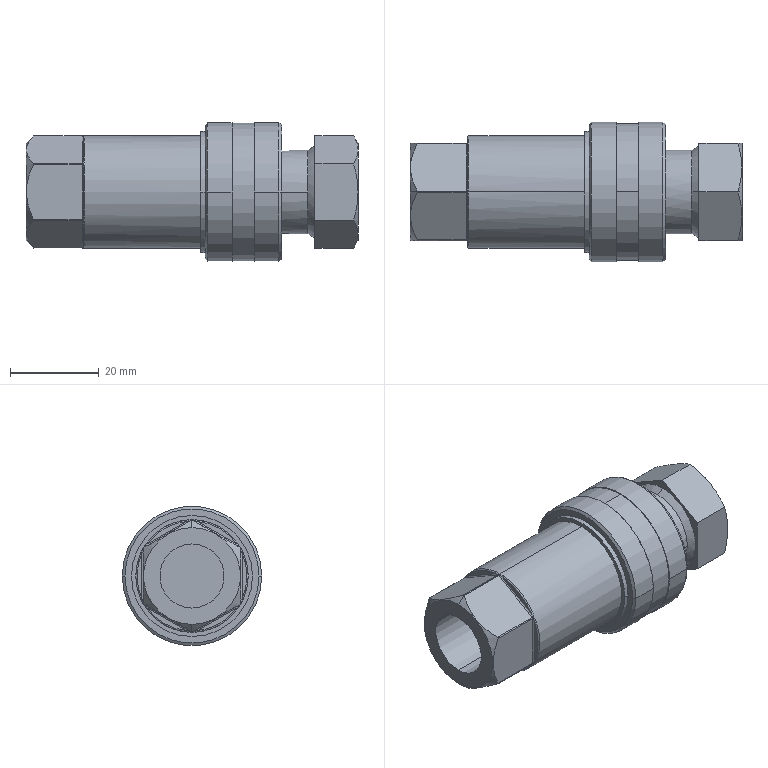Part | SolidWorks | features BaseBody 1 | 1 solid | 109 faces | box 75 x 31.5 x 31.5 mm | volume 35275 mm3 | cylinder 33 | spline 31 | plane 30 | cone 15 | commonest cylinder face diameters 0.6 x13 14.497 x4 31.5 x4 18.85 x2 25.403 x2 26.035 x2